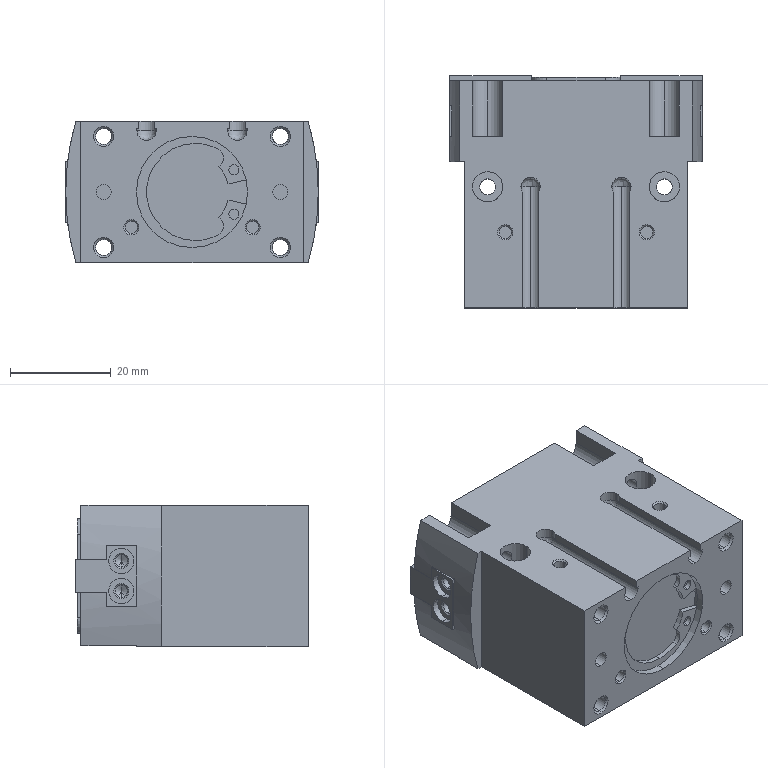Part | STEP file | 535861 HGPT-20-A---(asm_0)_5 | 4 solids | 340 faces | box 50 x 46 x 28 mm | volume 52148 mm3 | cylinder 140 | plane 114 | cone 84 | spline 2 | commonest cylinder face diameters 2.459 x34 3.2 x24 5 x16 6 x14 3.8 x10 3 x8